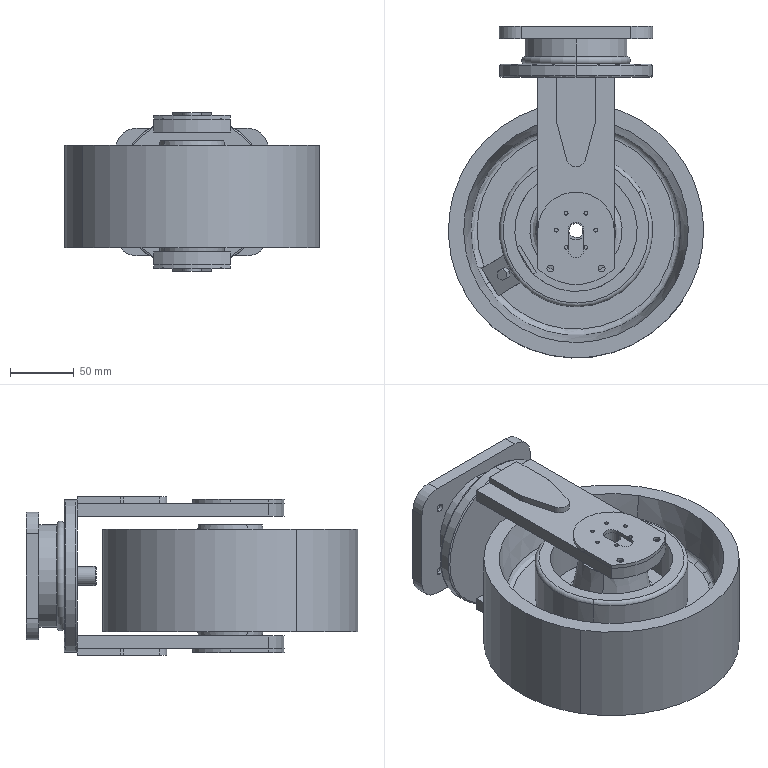Part | SolidWorks | features CompositeCurve 10, AEMSimFeature 1, MirrorCompFeat 1, ReferencePattern 1 | 5 solids | 252 faces | box 200 x 260 x 124 mm | volume 1930087 mm3 | cylinder 118 | plane 86 | cone 30 | torus 18 | commonest cylinder face diameters 3 x24 11 x19 5.5 x16 6.6 x8 15 x8 120 x6